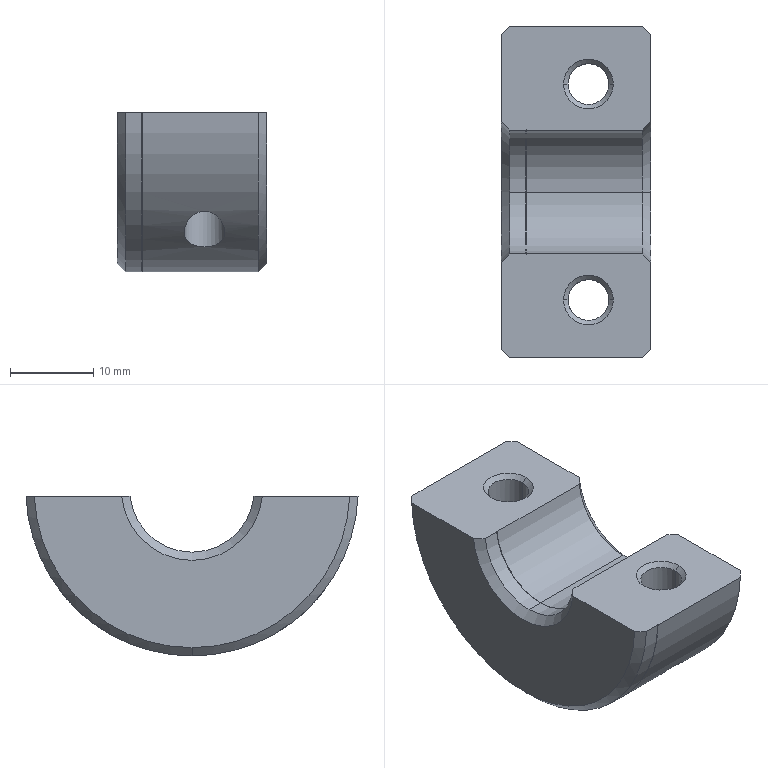Part | STEP file | 0232_Z_SSCSPD15_4 | 1 solid | 31 faces | box 18 x 39.974 x 19.251 mm | volume 8748 mm3 | cone 13 | cylinder 12 | plane 6 | commonest cylinder face diameters 4.917 x4 15 x4 40 x2 40.002 x2